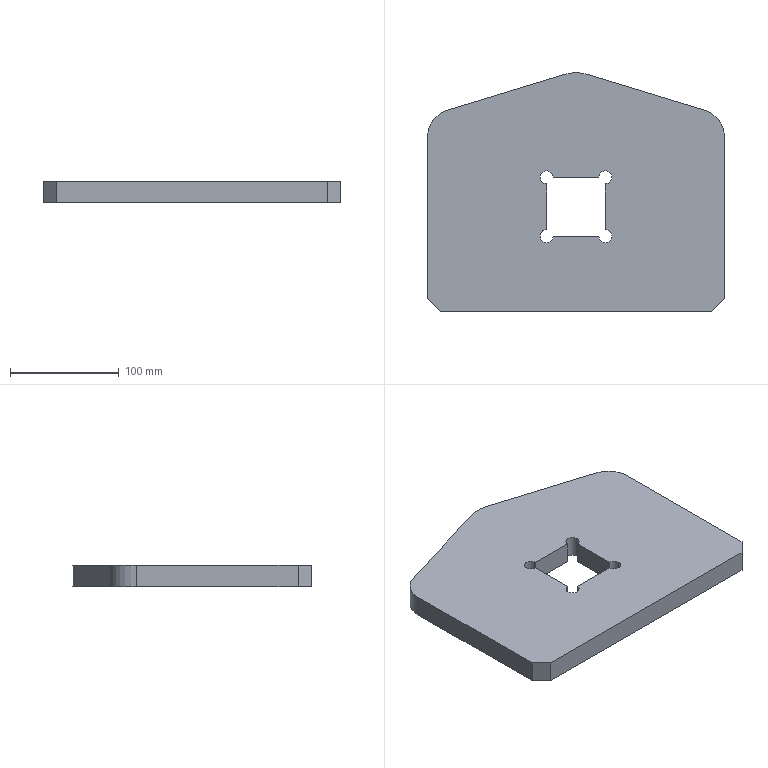Part | SolidWorks | features Extrusion 1 | 1 solid | 22 faces | box 273 x 219.3 x 20 mm | volume 1021205 mm3 | plane 13 | cylinder 9 | commonest cylinder face diameters 12 x6 50 x2 70 x1
STEP:
#1=CARTESIAN_POINT('',(-27.,75.,20.));
#2=VERTEX_POINT('',#1);
#3=CARTESIAN_POINT('',(-33.,69.,20.));
#4=VERTEX_POINT('',#3);
#5=CARTESIAN_POINT('',(-27.,69.,20.));
#6=DIRECTION('',(0.,0.,1.));
#7=DIRECTION('',(-1.,0.,0.));
#8=AXIS2_PLACEMENT_3D('',#5,#6,#7);
#9=CIRCLE('',#8,6.);
#10=EDGE_CURVE('',#2,#4,#9,.T.);
#11=ORIENTED_EDGE('',*,*,#10,.T.);
#12=CARTESIAN_POINT('',(-33.,69.,0.));
#13=VERTEX_POINT('',#12);
#14=CARTESIAN_POINT('',(-33.,69.,20.));
#15=DIRECTION('',(0.,0.,-1.));
#16=VECTOR('',#15,1000.);
#17=LINE('',#14,#16);
#18=EDGE_CURVE('',#4,#13,#17,.T.);
#19=ORIENTED_EDGE('',*,*,#18,.T.);
#20=CARTESIAN_POINT('',(-27.,75.,0.));
#21=VERTEX_POINT('',#20);
#22=CARTESIAN_POINT('',(-27.,69.,0.));
#23=DIRECTION('',(0.,0.,1.));
#24=DIRECTION('',(-1.,0.,0.));
#25=AXIS2_PLACEMENT_3D('',#22,#23,#24);
#26=CIRCLE('',#25,6.);
#27=EDGE_CURVE('',#21,#13,#26,.T.);
#28=ORIENTED_EDGE('',*,*,#27,.F.);
#29=CARTESIAN_POINT('',(-27.,75.,20.));
#30=DIRECTION('',(0.,0.,-1.));
#31=VECTOR('',#30,1000.);
#32=LINE('',#29,#31);
#33=EDGE_CURVE('',#2,#21,#32,.T.);
#34=ORIENTED_EDGE('',*,*,#33,.F.);
#35=EDGE_LOOP('',(#11,#19,#28,#34));
#36=FACE_OUTER_BOUND('',#35,.T.);
#37=CARTESIAN_POINT('',(-27.,69.,20.));
#38=DIRECTION('',(0.,0.,-1.));
#39=DIRECTION('',(-1.,0.,0.));
#40=AXIS2_PLACEMENT_3D('',#37,#38,#39);
#41=CYLINDRICAL_SURFACE('',#40,6.);
#42=ADVANCED_FACE('',(#36),#41,.F.);
#43=CARTESIAN_POINT('',(-21.,123.,20.));
#44=VERTEX_POINT('',#43);
#45=CARTESIAN_POINT('',(-33.,123.,20.));
#46=VERTEX_POINT('',#45);
#47=CARTESIAN_POINT('',(-27.,123.,20.));
#48=DIRECTION('',(0.,0.,1.));
#49=DIRECTION('',(-1.,0.,0.));
#50=AXIS2_PLACEMENT_3D('',#47,#48,#49);
#51=CIRCLE('',#50,6.);
#52=EDGE_CURVE('',#44,#46,#51,.T.);
#53=ORIENTED_EDGE('',*,*,#52,.T.);
#54=CARTESIAN_POINT('',(-33.,123.,0.));
#55=VERTEX_POINT('',#54);
#56=CARTESIAN_POINT('',(-33.,123.,20.));
#57=DIRECTION('',(0.,0.,-1.));
#58=VECTOR('',#57,1000.);
#59=LINE('',#56,#58);
#60=EDGE_CURVE('',#46,#55,#59,.T.);
#61=ORIENTED_EDGE('',*,*,#60,.T.);
#62=CARTESIAN_POINT('',(-21.,123.,0.));
#63=VERTEX_POINT('',#62);
#64=CARTESIAN_POINT('',(-27.,123.,0.));
#65=DIRECTION('',(0.,0.,1.));
#66=DIRECTION('',(-1.,0.,0.));
#67=AXIS2_PLACEMENT_3D('',#64,#65,#66);
#68=CIRCLE('',#67,6.);
#69=EDGE_CURVE('',#63,#55,#68,.T.);
#70=ORIENTED_EDGE('',*,*,#69,.F.);
#71=CARTESIAN_POINT('',(-21.,123.,20.));
#72=DIRECTION('',(0.,0.,-1.));
#73=VECTOR('',#72,1000.);
#74=LINE('',#71,#73);
#75=EDGE_CURVE('',#44,#63,#74,.T.);
#76=ORIENTED_EDGE('',*,*,#75,.F.);
#77=EDGE_LOOP('',(#53,#61,#70,#76));
#78=FACE_OUTER_BOUND('',#77,.T.);
#79=CARTESIAN_POINT('',(-27.,123.,20.));
#80=DIRECTION('',(0.,0.,-1.));
#81=DIRECTION('',(-1.,0.,0.));
#82=AXIS2_PLACEMENT_3D('',#79,#80,#81);
#83=CYLINDRICAL_SURFACE('',#82,6.);
#84=ADVANCED_FACE('',(#78),#83,.F.);
#85=CARTESIAN_POINT('',(124.5,0.,20.));
#86=VERTEX_POINT('',#85);
#87=CARTESIAN_POINT('',(136.5,12.,20.));
#88=VERTEX_POINT('',#87);
#89=CARTESIAN_POINT('',(124.5,0.,20.));
#90=DIRECTION('',(0.7071,0.7071,0.));
#91=VECTOR('',#90,1000.);
#92=LINE('',#89,#91);
#93=EDGE_CURVE('',#86,#88,#92,.T.);
#94=ORIENTED_EDGE('',*,*,#93,.T.);
#95=CARTESIAN_POINT('',(136.5,160.6,20.));
#96=VERTEX_POINT('',#95);
#97=CARTESIAN_POINT('',(136.5,12.,20.));
#98=DIRECTION('',(0.,1.,0.));
#99=VECTOR('',#98,1000.);
#100=LINE('',#97,#99);
#101=EDGE_CURVE('',#88,#96,#100,.T.);
#102=ORIENTED_EDGE('',*,*,#101,.T.);
#103=CARTESIAN_POINT('',(118.823,184.503,20.));
#104=VERTEX_POINT('',#103);
#105=CARTESIAN_POINT('',(111.5,160.6,20.));
#106=DIRECTION('',(0.,0.,1.));
#107=DIRECTION('',(1.,0.,0.));
#108=AXIS2_PLACEMENT_3D('',#105,#106,#107);
#109=CIRCLE('',#108,25.);
#110=EDGE_CURVE('',#96,#104,#109,.T.);
#111=ORIENTED_EDGE('',*,*,#110,.T.);
#112=CARTESIAN_POINT('',(10.252,217.765,20.));
#113=VERTEX_POINT('',#112);
#114=CARTESIAN_POINT('',(10.252,217.765,20.));
#115=DIRECTION('',(-0.9561,0.2929,0.));
#116=VECTOR('',#115,1000.);
#117=LINE('',#114,#116);
#118=EDGE_CURVE('',#104,#113,#117,.T.);
#119=ORIENTED_EDGE('',*,*,#118,.T.);
#120=CARTESIAN_POINT('',(-10.252,217.765,20.));
#121=VERTEX_POINT('',#120);
#122=CARTESIAN_POINT('',(0.,184.3,20.));
#123=DIRECTION('',(0.,0.,1.));
#124=DIRECTION('',(1.,0.,0.));
#125=AXIS2_PLACEMENT_3D('',#122,#123,#124);
#126=CIRCLE('',#125,35.);
#127=EDGE_CURVE('',#113,#121,#126,.T.);
#128=ORIENTED_EDGE('',*,*,#127,.T.);
#129=CARTESIAN_POINT('',(-118.823,184.503,20.));
#130=VERTEX_POINT('',#129);
#131=CARTESIAN_POINT('',(-10.252,217.765,20.));
#132=DIRECTION('',(-0.9561,-0.2929,0.));
#133=VECTOR('',#132,1000.);
#134=LINE('',#131,#133);
#135=EDGE_CURVE('',#121,#130,#134,.T.);
#136=ORIENTED_EDGE('',*,*,#135,.T.);
#137=CARTESIAN_POINT('',(-136.5,160.6,20.));
#138=VERTEX_POINT('',#137);
#139=CARTESIAN_POINT('',(-111.5,160.6,20.));
#140=DIRECTION('',(0.,0.,1.));
#141=DIRECTION('',(-1.,0.,0.));
#142=AXIS2_PLACEMENT_3D('',#139,#140,#141);
#143=CIRCLE('',#142,25.);
#144=EDGE_CURVE('',#130,#138,#143,.T.);
#145=ORIENTED_EDGE('',*,*,#144,.T.);
#146=CARTESIAN_POINT('',(-136.5,12.,20.));
#147=VERTEX_POINT('',#146);
#148=CARTESIAN_POINT('',(-136.5,12.,20.));
#149=DIRECTION('',(0.,-1.,0.));
#150=VECTOR('',#149,1000.);
#151=LINE('',#148,#150);
#152=EDGE_CURVE('',#138,#147,#151,.T.);
#153=ORIENTED_EDGE('',*,*,#152,.T.);
#154=CARTESIAN_POINT('',(-124.5,0.,20.));
#155=VERTEX_POINT('',#154);
#156=CARTESIAN_POINT('',(-124.5,0.,20.));
#157=DIRECTION('',(0.7071,-0.7071,0.));
#158=VECTOR('',#157,1000.);
#159=LINE('',#156,#158);
#160=EDGE_CURVE('',#147,#155,#159,.T.);
#161=ORIENTED_EDGE('',*,*,#160,.T.);
#162=CARTESIAN_POINT('',(-124.5,0.,20.));
#163=DIRECTION('',(1.,0.,0.));
#164=VECTOR('',#163,1000.);
#165=LINE('',#162,#164);
#166=EDGE_CURVE('',#155,#86,#165,.T.);
#167=ORIENTED_EDGE('',*,*,#166,.T.);
#168=EDGE_LOOP('',(#94,#102,#111,#119,#128,#136,#145,#153,#161,#167));
#169=FACE_OUTER_BOUND('',#168,.T.);
#170=CARTESIAN_POINT('',(27.,75.,20.));
#171=VERTEX_POINT('',#170);
#172=CARTESIAN_POINT('',(27.,117.,20.));
#173=VERTEX_POINT('',#172);
#174=CARTESIAN_POINT('',(27.,117.,20.));
#175=DIRECTION('',(0.,1.,0.));
#176=VECTOR('',#175,1000.);
#177=LINE('',#174,#176);
#178=EDGE_CURVE('',#171,#173,#177,.T.);
#179=ORIENTED_EDGE('',*,*,#178,.F.);
#180=CARTESIAN_POINT('',(21.,69.,20.));
#181=VERTEX_POINT('',#180);
#182=CARTESIAN_POINT('',(27.,69.,20.));
#183=DIRECTION('',(0.,0.,1.));
#184=DIRECTION('',(1.,0.,0.));
#185=AXIS2_PLACEMENT_3D('',#182,#183,#184);
#186=CIRCLE('',#185,6.);
#187=EDGE_CURVE('',#181,#171,#186,.T.);
#188=ORIENTED_EDGE('',*,*,#187,.F.);
#189=CARTESIAN_POINT('',(-21.,69.,20.));
#190=VERTEX_POINT('',#189);
#191=CARTESIAN_POINT('',(21.,69.,20.));
#192=DIRECTION('',(1.,0.,0.));
#193=VECTOR('',#192,1000.);
#194=LINE('',#191,#193);
#195=EDGE_CURVE('',#190,#181,#194,.T.);
#196=ORIENTED_EDGE('',*,*,#195,.F.);
#197=CARTESIAN_POINT('',(-27.,69.,20.));
#198=DIRECTION('',(0.,0.,1.));
#199=DIRECTION('',(-1.,0.,0.));
#200=AXIS2_PLACEMENT_3D('',#197,#198,#199);
#201=CIRCLE('',#200,6.);
#202=EDGE_CURVE('',#4,#190,#201,.T.);
#203=ORIENTED_EDGE('',*,*,#202,.F.);
#204=ORIENTED_EDGE('',*,*,#10,.F.);
#205=CARTESIAN_POINT('',(-27.,117.,20.));
#206=VERTEX_POINT('',#205);
#207=CARTESIAN_POINT('',(-27.,117.,20.));
#208=DIRECTION('',(0.,-1.,0.));
#209=VECTOR('',#208,1000.);
#210=LINE('',#207,#209);
#211=EDGE_CURVE('',#206,#2,#210,.T.);
#212=ORIENTED_EDGE('',*,*,#211,.F.);
#213=CARTESIAN_POINT('',(-27.,123.,20.));
#214=DIRECTION('',(0.,0.,1.));
#215=DIRECTION('',(-1.,0.,0.));
#216=AXIS2_PLACEMENT_3D('',#213,#214,#215);
#217=CIRCLE('',#216,6.);
#218=EDGE_CURVE('',#46,#206,#217,.T.);
#219=ORIENTED_EDGE('',*,*,#218,.F.);
#220=ORIENTED_EDGE('',*,*,#52,.F.);
#221=CARTESIAN_POINT('',(21.,123.,20.));
#222=VERTEX_POINT('',#221);
#223=CARTESIAN_POINT('',(-21.,123.,20.));
#224=DIRECTION('',(-1.,0.,0.));
#225=VECTOR('',#224,1000.);
#226=LINE('',#223,#225);
#227=EDGE_CURVE('',#222,#44,#226,.T.);
#228=ORIENTED_EDGE('',*,*,#227,.F.);
#229=CARTESIAN_POINT('',(27.,123.,20.));
#230=DIRECTION('',(0.,0.,1.));
#231=DIRECTION('',(1.,0.,0.));
#232=AXIS2_PLACEMENT_3D('',#229,#230,#231);
#233=CIRCLE('',#232,6.);
#234=EDGE_CURVE('',#173,#222,#233,.T.);
#235=ORIENTED_EDGE('',*,*,#234,.F.);
#236=EDGE_LOOP('',(#179,#188,#196,#203,#204,#212,#219,#220,#228,#235));
#237=FACE_BOUND('',#236,.T.);
#238=CARTESIAN_POINT('',(111.5,160.6,20.));
#239=DIRECTION('',(0.,0.,1.));
#240=DIRECTION('',(1.,0.,0.));
#241=AXIS2_PLACEMENT_3D('',#238,#239,#240);
#242=PLANE('',#241);
#243=ADVANCED_FACE('',(#169,#237),#242,.T.);
#244=CARTESIAN_POINT('',(124.5,0.,0.));
#245=VERTEX_POINT('',#244);
#246=CARTESIAN_POINT('',(136.5,12.,0.));
#247=VERTEX_POINT('',#246);
#248=CARTESIAN_POINT('',(124.5,0.,0.));
#249=DIRECTION('',(0.7071,0.7071,0.));
#250=VECTOR('',#249,1000.);
#251=LINE('',#248,#250);
#252=EDGE_CURVE('',#245,#247,#251,.T.);
#253=ORIENTED_EDGE('',*,*,#252,.F.);
#254=CARTESIAN_POINT('',(-124.5,0.,0.));
#255=VERTEX_POINT('',#254);
#256=CARTESIAN_POINT('',(-124.5,0.,0.));
#257=DIRECTION('',(1.,0.,0.));
#258=VECTOR('',#257,1000.);
#259=LINE('',#256,#258);
#260=EDGE_CURVE('',#255,#245,#259,.T.);
#261=ORIENTED_EDGE('',*,*,#260,.F.);
#262=CARTESIAN_POINT('',(-136.5,12.,0.));
#263=VERTEX_POINT('',#262);
#264=CARTESIAN_POINT('',(-124.5,0.,0.));
#265=DIRECTION('',(0.7071,-0.7071,0.));
#266=VECTOR('',#265,1000.);
#267=LINE('',#264,#266);
#268=EDGE_CURVE('',#263,#255,#267,.T.);
#269=ORIENTED_EDGE('',*,*,#268,.F.);
#270=CARTESIAN_POINT('',(-136.5,160.6,0.));
#271=VERTEX_POINT('',#270);
#272=CARTESIAN_POINT('',(-136.5,12.,0.));
#273=DIRECTION('',(0.,-1.,0.));
#274=VECTOR('',#273,1000.);
#275=LINE('',#272,#274);
#276=EDGE_CURVE('',#271,#263,#275,.T.);
#277=ORIENTED_EDGE('',*,*,#276,.F.);
#278=CARTESIAN_POINT('',(-118.823,184.503,0.));
#279=VERTEX_POINT('',#278);
#280=CARTESIAN_POINT('',(-111.5,160.6,0.));
#281=DIRECTION('',(0.,0.,1.));
#282=DIRECTION('',(-1.,0.,0.));
#283=AXIS2_PLACEMENT_3D('',#280,#281,#282);
#284=CIRCLE('',#283,25.);
#285=EDGE_CURVE('',#279,#271,#284,.T.);
#286=ORIENTED_EDGE('',*,*,#285,.F.);
#287=CARTESIAN_POINT('',(-10.252,217.765,0.));
#288=VERTEX_POINT('',#287);
#289=CARTESIAN_POINT('',(-10.252,217.765,0.));
#290=DIRECTION('',(-0.9561,-0.2929,0.));
#291=VECTOR('',#290,1000.);
#292=LINE('',#289,#291);
#293=EDGE_CURVE('',#288,#279,#292,.T.);
#294=ORIENTED_EDGE('',*,*,#293,.F.);
#295=CARTESIAN_POINT('',(10.252,217.765,0.));
#296=VERTEX_POINT('',#295);
#297=CARTESIAN_POINT('',(0.,184.3,0.));
#298=DIRECTION('',(0.,0.,1.));
#299=DIRECTION('',(1.,0.,0.));
#300=AXIS2_PLACEMENT_3D('',#297,#298,#299);
#301=CIRCLE('',#300,35.);
#302=EDGE_CURVE('',#296,#288,#301,.T.);
#303=ORIENTED_EDGE('',*,*,#302,.F.);
#304=CARTESIAN_POINT('',(118.823,184.503,0.));
#305=VERTEX_POINT('',#304);
#306=CARTESIAN_POINT('',(10.252,217.765,0.));
#307=DIRECTION('',(-0.9561,0.2929,0.));
#308=VECTOR('',#307,1000.);
#309=LINE('',#306,#308);
#310=EDGE_CURVE('',#305,#296,#309,.T.);
#311=ORIENTED_EDGE('',*,*,#310,.F.);
#312=CARTESIAN_POINT('',(136.5,160.6,0.));
#313=VERTEX_POINT('',#312);
#314=CARTESIAN_POINT('',(111.5,160.6,0.));
#315=DIRECTION('',(0.,0.,1.));
#316=DIRECTION('',(1.,0.,0.));
#317=AXIS2_PLACEMENT_3D('',#314,#315,#316);
#318=CIRCLE('',#317,25.);
#319=EDGE_CURVE('',#313,#305,#318,.T.);
#320=ORIENTED_EDGE('',*,*,#319,.F.);
#321=CARTESIAN_POINT('',(136.5,12.,0.));
#322=DIRECTION('',(0.,1.,0.));
#323=VECTOR('',#322,1000.);
#324=LINE('',#321,#323);
#325=EDGE_CURVE('',#247,#313,#324,.T.);
#326=ORIENTED_EDGE('',*,*,#325,.F.);
#327=EDGE_LOOP('',(#253,#261,#269,#277,#286,#294,#303,#311,#320,#326));
#328=FACE_OUTER_BOUND('',#327,.T.);
#329=CARTESIAN_POINT('',(21.,69.,0.));
#330=VERTEX_POINT('',#329);
#331=CARTESIAN_POINT('',(27.,75.,0.));
#332=VERTEX_POINT('',#331);
#333=CARTESIAN_POINT('',(27.,69.,0.));
#334=DIRECTION('',(0.,0.,1.));
#335=DIRECTION('',(1.,0.,0.));
#336=AXIS2_PLACEMENT_3D('',#333,#334,#335);
#337=CIRCLE('',#336,6.);
#338=EDGE_CURVE('',#330,#332,#337,.T.);
#339=ORIENTED_EDGE('',*,*,#338,.T.);
#340=CARTESIAN_POINT('',(27.,117.,0.));
#341=VERTEX_POINT('',#340);
#342=CARTESIAN_POINT('',(27.,117.,0.));
#343=DIRECTION('',(0.,1.,0.));
#344=VECTOR('',#343,1000.);
#345=LINE('',#342,#344);
#346=EDGE_CURVE('',#332,#341,#345,.T.);
#347=ORIENTED_EDGE('',*,*,#346,.T.);
#348=CARTESIAN_POINT('',(21.,123.,0.));
#349=VERTEX_POINT('',#348);
#350=CARTESIAN_POINT('',(27.,123.,0.));
#351=DIRECTION('',(0.,0.,1.));
#352=DIRECTION('',(1.,0.,0.));
#353=AXIS2_PLACEMENT_3D('',#350,#351,#352);
#354=CIRCLE('',#353,6.);
#355=EDGE_CURVE('',#341,#349,#354,.T.);
#356=ORIENTED_EDGE('',*,*,#355,.T.);
#357=CARTESIAN_POINT('',(-21.,123.,0.));
#358=DIRECTION('',(-1.,0.,0.));
#359=VECTOR('',#358,1000.);
#360=LINE('',#357,#359);
#361=EDGE_CURVE('',#349,#63,#360,.T.);
#362=ORIENTED_EDGE('',*,*,#361,.T.);
#363=ORIENTED_EDGE('',*,*,#69,.T.);
#364=CARTESIAN_POINT('',(-27.,117.,0.));
#365=VERTEX_POINT('',#364);
#366=CARTESIAN_POINT('',(-27.,123.,0.));
#367=DIRECTION('',(0.,0.,1.));
#368=DIRECTION('',(-1.,0.,0.));
#369=AXIS2_PLACEMENT_3D('',#366,#367,#368);
#370=CIRCLE('',#369,6.);
#371=EDGE_CURVE('',#55,#365,#370,.T.);
#372=ORIENTED_EDGE('',*,*,#371,.T.);
#373=CARTESIAN_POINT('',(-27.,117.,0.));
#374=DIRECTION('',(0.,-1.,0.));
#375=VECTOR('',#374,1000.);
#376=LINE('',#373,#375);
#377=EDGE_CURVE('',#365,#21,#376,.T.);
#378=ORIENTED_EDGE('',*,*,#377,.T.);
#379=ORIENTED_EDGE('',*,*,#27,.T.);
#380=CARTESIAN_POINT('',(-21.,69.,0.));
#381=VERTEX_POINT('',#380);
#382=CARTESIAN_POINT('',(-27.,69.,0.));
#383=DIRECTION('',(0.,0.,1.));
#384=DIRECTION('',(-1.,0.,0.));
#385=AXIS2_PLACEMENT_3D('',#382,#383,#384);
#386=CIRCLE('',#385,6.);
#387=EDGE_CURVE('',#13,#381,#386,.T.);
#388=ORIENTED_EDGE('',*,*,#387,.T.);
#389=CARTESIAN_POINT('',(21.,69.,0.));
#390=DIRECTION('',(1.,0.,0.));
#391=VECTOR('',#390,1000.);
#392=LINE('',#389,#391);
#393=EDGE_CURVE('',#381,#330,#392,.T.);
#394=ORIENTED_EDGE('',*,*,#393,.T.);
#395=EDGE_LOOP('',(#339,#347,#356,#362,#363,#372,#378,#379,#388,#394));
#396=FACE_BOUND('',#395,.T.);
#397=CARTESIAN_POINT('',(111.5,160.6,0.));
#398=DIRECTION('',(0.,0.,1.));
#399=DIRECTION('',(1.,0.,0.));
#400=AXIS2_PLACEMENT_3D('',#397,#398,#399);
#401=PLANE('',#400);
#402=ADVANCED_FACE('',(#328,#396),#401,.F.);
#403=ORIENTED_EDGE('',*,*,#252,.T.);
#404=CARTESIAN_POINT('',(136.5,12.,20.));
#405=DIRECTION('',(0.,0.,-1.));
#406=VECTOR('',#405,1000.);
#407=LINE('',#404,#406);
#408=EDGE_CURVE('',#88,#247,#407,.T.);
#409=ORIENTED_EDGE('',*,*,#408,.F.);
#410=ORIENTED_EDGE('',*,*,#93,.F.);
#411=CARTESIAN_POINT('',(124.5,0.,20.));
#412=DIRECTION('',(0.,0.,-1.));
#413=VECTOR('',#412,1000.);
#414=LINE('',#411,#413);
#415=EDGE_CURVE('',#86,#245,#414,.T.);
#416=ORIENTED_EDGE('',*,*,#415,.T.);
#417=EDGE_LOOP('',(#403,#409,#410,#416));
#418=FACE_OUTER_BOUND('',#417,.T.);
#419=CARTESIAN_POINT('',(124.5,0.,20.));
#420=DIRECTION('',(-0.7071,0.7071,0.));
#421=DIRECTION('',(-0.7071,-0.7071,0.));
#422=AXIS2_PLACEMENT_3D('',#419,#420,#421);
#423=PLANE('',#422);
#424=ADVANCED_FACE('',(#418),#423,.F.);
#425=ORIENTED_EDGE('',*,*,#325,.T.);
#426=CARTESIAN_POINT('',(136.5,160.6,20.));
#427=DIRECTION('',(0.,0.,-1.));
#428=VECTOR('',#427,1000.);
#429=LINE('',#426,#428);
#430=EDGE_CURVE('',#96,#313,#429,.T.);
#431=ORIENTED_EDGE('',*,*,#430,.F.);
#432=ORIENTED_EDGE('',*,*,#101,.F.);
#433=ORIENTED_EDGE('',*,*,#408,.T.);
#434=EDGE_LOOP('',(#425,#431,#432,#433));
#435=FACE_OUTER_BOUND('',#434,.T.);
#436=CARTESIAN_POINT('',(136.5,12.,20.));
#437=DIRECTION('',(-1.,0.,0.));
#438=DIRECTION('',(0.,0.,1.));
#439=AXIS2_PLACEMENT_3D('',#436,#437,#438);
#440=PLANE('',#439);
#441=ADVANCED_FACE('',(#435),#440,.F.);
#442=ORIENTED_EDGE('',*,*,#319,.T.);
#443=CARTESIAN_POINT('',(118.823,184.503,20.));
#444=DIRECTION('',(0.,0.,-1.));
#445=VECTOR('',#444,1000.);
#446=LINE('',#443,#445);
#447=EDGE_CURVE('',#104,#305,#446,.T.);
#448=ORIENTED_EDGE('',*,*,#447,.F.);
#449=ORIENTED_EDGE('',*,*,#110,.F.);
#450=ORIENTED_EDGE('',*,*,#430,.T.);
#451=EDGE_LOOP('',(#442,#448,#449,#450));
#452=FACE_OUTER_BOUND('',#451,.T.);
#453=CARTESIAN_POINT('',(111.5,160.6,20.));
#454=DIRECTION('',(0.,0.,-1.));
#455=DIRECTION('',(-1.,0.,0.));
#456=AXIS2_PLACEMENT_3D('',#453,#454,#455);
#457=CYLINDRICAL_SURFACE('',#456,25.);
#458=ADVANCED_FACE('',(#452),#457,.T.);
#459=ORIENTED_EDGE('',*,*,#310,.T.);
#460=CARTESIAN_POINT('',(10.252,217.765,20.));
#461=DIRECTION('',(0.,0.,-1.));
#462=VECTOR('',#461,1000.);
#463=LINE('',#460,#462);
#464=EDGE_CURVE('',#113,#296,#463,.T.);
#465=ORIENTED_EDGE('',*,*,#464,.F.);
#466=ORIENTED_EDGE('',*,*,#118,.F.);
#467=ORIENTED_EDGE('',*,*,#447,.T.);
#468=EDGE_LOOP('',(#459,#465,#466,#467));
#469=FACE_OUTER_BOUND('',#468,.T.);
#470=CARTESIAN_POINT('',(10.252,217.765,20.));
#471=DIRECTION('',(-0.2929,-0.9561,0.));
#472=DIRECTION('',(0.9561,-0.2929,0.));
#473=AXIS2_PLACEMENT_3D('',#470,#471,#472);
#474=PLANE('',#473);
#475=ADVANCED_FACE('',(#469),#474,.F.);
#476=ORIENTED_EDGE('',*,*,#302,.T.);
#477=CARTESIAN_POINT('',(-10.252,217.765,20.));
#478=DIRECTION('',(0.,0.,-1.));
#479=VECTOR('',#478,1000.);
#480=LINE('',#477,#479);
#481=EDGE_CURVE('',#121,#288,#480,.T.);
#482=ORIENTED_EDGE('',*,*,#481,.F.);
#483=ORIENTED_EDGE('',*,*,#127,.F.);
#484=ORIENTED_EDGE('',*,*,#464,.T.);
#485=EDGE_LOOP('',(#476,#482,#483,#484));
#486=FACE_OUTER_BOUND('',#485,.T.);
#487=CARTESIAN_POINT('',(0.,184.3,20.));
#488=DIRECTION('',(0.,0.,-1.));
#489=DIRECTION('',(-1.,0.,0.));
#490=AXIS2_PLACEMENT_3D('',#487,#488,#489);
#491=CYLINDRICAL_SURFACE('',#490,35.);
#492=ADVANCED_FACE('',(#486),#491,.T.);
#493=ORIENTED_EDGE('',*,*,#293,.T.);
#494=CARTESIAN_POINT('',(-118.823,184.503,20.));
#495=DIRECTION('',(0.,0.,-1.));
#496=VECTOR('',#495,1000.);
#497=LINE('',#494,#496);
#498=EDGE_CURVE('',#130,#279,#497,.T.);
#499=ORIENTED_EDGE('',*,*,#498,.F.);
#500=ORIENTED_EDGE('',*,*,#135,.F.);
#501=ORIENTED_EDGE('',*,*,#481,.T.);
#502=EDGE_LOOP('',(#493,#499,#500,#501));
#503=FACE_OUTER_BOUND('',#502,.T.);
#504=CARTESIAN_POINT('',(-10.252,217.765,20.));
#505=DIRECTION('',(0.2929,-0.9561,0.));
#506=DIRECTION('',(0.9561,0.2929,0.));
#507=AXIS2_PLACEMENT_3D('',#504,#505,#506);
#508=PLANE('',#507);
#509=ADVANCED_FACE('',(#503),#508,.F.);
#510=ORIENTED_EDGE('',*,*,#285,.T.);
#511=CARTESIAN_POINT('',(-136.5,160.6,20.));
#512=DIRECTION('',(0.,0.,-1.));
#513=VECTOR('',#512,1000.);
#514=LINE('',#511,#513);
#515=EDGE_CURVE('',#138,#271,#514,.T.);
#516=ORIENTED_EDGE('',*,*,#515,.F.);
#517=ORIENTED_EDGE('',*,*,#144,.F.);
#518=ORIENTED_EDGE('',*,*,#498,.T.);
#519=EDGE_LOOP('',(#510,#516,#517,#518));
#520=FACE_OUTER_BOUND('',#519,.T.);
#521=CARTESIAN_POINT('',(-111.5,160.6,20.));
#522=DIRECTION('',(0.,0.,-1.));
#523=DIRECTION('',(-1.,0.,0.));
#524=AXIS2_PLACEMENT_3D('',#521,#522,#523);
#525=CYLINDRICAL_SURFACE('',#524,25.);
#526=ADVANCED_FACE('',(#520),#525,.T.);
#527=ORIENTED_EDGE('',*,*,#276,.T.);
#528=CARTESIAN_POINT('',(-136.5,12.,20.));
#529=DIRECTION('',(0.,0.,-1.));
#530=VECTOR('',#529,1000.);
#531=LINE('',#528,#530);
#532=EDGE_CURVE('',#147,#263,#531,.T.);
#533=ORIENTED_EDGE('',*,*,#532,.F.);
#534=ORIENTED_EDGE('',*,*,#152,.F.);
#535=ORIENTED_EDGE('',*,*,#515,.T.);
#536=EDGE_LOOP('',(#527,#533,#534,#535));
#537=FACE_OUTER_BOUND('',#536,.T.);
#538=CARTESIAN_POINT('',(-136.5,12.,20.));
#539=DIRECTION('',(1.,0.,0.));
#540=DIRECTION('',(0.,0.,-1.));
#541=AXIS2_PLACEMENT_3D('',#538,#539,#540);
#542=PLANE('',#541);
#543=ADVANCED_FACE('',(#537),#542,.F.);
#544=ORIENTED_EDGE('',*,*,#268,.T.);
#545=CARTESIAN_POINT('',(-124.5,0.,20.));
#546=DIRECTION('',(0.,0.,-1.));
#547=VECTOR('',#546,1000.);
#548=LINE('',#545,#547);
#549=EDGE_CURVE('',#155,#255,#548,.T.);
#550=ORIENTED_EDGE('',*,*,#549,.F.);
#551=ORIENTED_EDGE('',*,*,#160,.F.);
#552=ORIENTED_EDGE('',*,*,#532,.T.);
#553=EDGE_LOOP('',(#544,#550,#551,#552));
#554=FACE_OUTER_BOUND('',#553,.T.);
#555=CARTESIAN_POINT('',(-124.5,0.,20.));
#556=DIRECTION('',(0.7071,0.7071,0.));
#557=DIRECTION('',(-0.7071,0.7071,0.));
#558=AXIS2_PLACEMENT_3D('',#555,#556,#557);
#559=PLANE('',#558);
#560=ADVANCED_FACE('',(#554),#559,.F.);
#561=ORIENTED_EDGE('',*,*,#260,.T.);
#562=ORIENTED_EDGE('',*,*,#415,.F.);
#563=ORIENTED_EDGE('',*,*,#166,.F.);
#564=ORIENTED_EDGE('',*,*,#549,.T.);
#565=EDGE_LOOP('',(#561,#562,#563,#564));
#566=FACE_OUTER_BOUND('',#565,.T.);
#567=CARTESIAN_POINT('',(-124.5,0.,20.));
#568=DIRECTION('',(0.,1.,0.));
#569=DIRECTION('',(0.,0.,1.));
#570=AXIS2_PLACEMENT_3D('',#567,#568,#569);
#571=PLANE('',#570);
#572=ADVANCED_FACE('',(#566),#571,.F.);
#573=ORIENTED_EDGE('',*,*,#338,.F.);
#574=CARTESIAN_POINT('',(21.,69.,20.));
#575=DIRECTION('',(0.,0.,-1.));
#576=VECTOR('',#575,1000.);
#577=LINE('',#574,#576);
#578=EDGE_CURVE('',#181,#330,#577,.T.);
#579=ORIENTED_EDGE('',*,*,#578,.F.);
#580=ORIENTED_EDGE('',*,*,#187,.T.);
#581=CARTESIAN_POINT('',(27.,75.,20.));
#582=DIRECTION('',(0.,0.,-1.));
#583=VECTOR('',#582,1000.);
#584=LINE('',#581,#583);
#585=EDGE_CURVE('',#171,#332,#584,.T.);
#586=ORIENTED_EDGE('',*,*,#585,.T.);
#587=EDGE_LOOP('',(#573,#579,#580,#586));
#588=FACE_OUTER_BOUND('',#587,.T.);
#589=CARTESIAN_POINT('',(27.,69.,20.));
#590=DIRECTION('',(0.,0.,-1.));
#591=DIRECTION('',(-1.,0.,0.));
#592=AXIS2_PLACEMENT_3D('',#589,#590,#591);
#593=CYLINDRICAL_SURFACE('',#592,6.);
#594=ADVANCED_FACE('',(#588),#593,.F.);
#595=ORIENTED_EDGE('',*,*,#346,.F.);
#596=ORIENTED_EDGE('',*,*,#585,.F.);
#597=ORIENTED_EDGE('',*,*,#178,.T.);
#598=CARTESIAN_POINT('',(27.,117.,20.));
#599=DIRECTION('',(0.,0.,-1.));
#600=VECTOR('',#599,1000.);
#601=LINE('',#598,#600);
#602=EDGE_CURVE('',#173,#341,#601,.T.);
#603=ORIENTED_EDGE('',*,*,#602,.T.);
#604=EDGE_LOOP('',(#595,#596,#597,#603));
#605=FACE_OUTER_BOUND('',#604,.T.);
#606=CARTESIAN_POINT('',(27.,117.,20.));
#607=DIRECTION('',(-1.,0.,0.));
#608=DIRECTION('',(0.,-1.,0.));
#609=AXIS2_PLACEMENT_3D('',#606,#607,#608);
#610=PLANE('',#609);
#611=ADVANCED_FACE('',(#605),#610,.T.);
#612=ORIENTED_EDGE('',*,*,#355,.F.);
#613=ORIENTED_EDGE('',*,*,#602,.F.);
#614=ORIENTED_EDGE('',*,*,#234,.T.);
#615=CARTESIAN_POINT('',(21.,123.,20.));
#616=DIRECTION('',(0.,0.,-1.));
#617=VECTOR('',#616,1000.);
#618=LINE('',#615,#617);
#619=EDGE_CURVE('',#222,#349,#618,.T.);
#620=ORIENTED_EDGE('',*,*,#619,.T.);
#621=EDGE_LOOP('',(#612,#613,#614,#620));
#622=FACE_OUTER_BOUND('',#621,.T.);
#623=CARTESIAN_POINT('',(27.,123.,20.));
#624=DIRECTION('',(0.,0.,-1.));
#625=DIRECTION('',(-1.,0.,0.));
#626=AXIS2_PLACEMENT_3D('',#623,#624,#625);
#627=CYLINDRICAL_SURFACE('',#626,6.);
#628=ADVANCED_FACE('',(#622),#627,.F.);
#629=ORIENTED_EDGE('',*,*,#361,.F.);
#630=ORIENTED_EDGE('',*,*,#619,.F.);
#631=ORIENTED_EDGE('',*,*,#227,.T.);
#632=ORIENTED_EDGE('',*,*,#75,.T.);
#633=EDGE_LOOP('',(#629,#630,#631,#632));
#634=FACE_OUTER_BOUND('',#633,.T.);
#635=CARTESIAN_POINT('',(-21.,123.,20.));
#636=DIRECTION('',(0.,-1.,0.));
#637=DIRECTION('',(0.,0.,-1.));
#638=AXIS2_PLACEMENT_3D('',#635,#636,#637);
#639=PLANE('',#638);
#640=ADVANCED_FACE('',(#634),#639,.T.);
#641=ORIENTED_EDGE('',*,*,#60,.F.);
#642=ORIENTED_EDGE('',*,*,#218,.T.);
#643=CARTESIAN_POINT('',(-27.,117.,20.));
#644=DIRECTION('',(0.,0.,-1.));
#645=VECTOR('',#644,1000.);
#646=LINE('',#643,#645);
#647=EDGE_CURVE('',#206,#365,#646,.T.);
#648=ORIENTED_EDGE('',*,*,#647,.T.);
#649=ORIENTED_EDGE('',*,*,#371,.F.);
#650=EDGE_LOOP('',(#641,#642,#648,#649));
#651=FACE_OUTER_BOUND('',#650,.T.);
#652=CARTESIAN_POINT('',(-27.,123.,20.));
#653=DIRECTION('',(0.,0.,-1.));
#654=DIRECTION('',(-1.,0.,0.));
#655=AXIS2_PLACEMENT_3D('',#652,#653,#654);
#656=CYLINDRICAL_SURFACE('',#655,6.);
#657=ADVANCED_FACE('',(#651),#656,.F.);
#658=ORIENTED_EDGE('',*,*,#377,.F.);
#659=ORIENTED_EDGE('',*,*,#647,.F.);
#660=ORIENTED_EDGE('',*,*,#211,.T.);
#661=ORIENTED_EDGE('',*,*,#33,.T.);
#662=EDGE_LOOP('',(#658,#659,#660,#661));
#663=FACE_OUTER_BOUND('',#662,.T.);
#664=CARTESIAN_POINT('',(-27.,117.,20.));
#665=DIRECTION('',(1.,0.,0.));
#666=DIRECTION('',(0.,1.,0.));
#667=AXIS2_PLACEMENT_3D('',#664,#665,#666);
#668=PLANE('',#667);
#669=ADVANCED_FACE('',(#663),#668,.T.);
#670=ORIENTED_EDGE('',*,*,#18,.F.);
#671=ORIENTED_EDGE('',*,*,#202,.T.);
#672=CARTESIAN_POINT('',(-21.,69.,20.));
#673=DIRECTION('',(0.,0.,-1.));
#674=VECTOR('',#673,1000.);
#675=LINE('',#672,#674);
#676=EDGE_CURVE('',#190,#381,#675,.T.);
#677=ORIENTED_EDGE('',*,*,#676,.T.);
#678=ORIENTED_EDGE('',*,*,#387,.F.);
#679=EDGE_LOOP('',(#670,#671,#677,#678));
#680=FACE_OUTER_BOUND('',#679,.T.);
#681=CARTESIAN_POINT('',(-27.,69.,20.));
#682=DIRECTION('',(0.,0.,-1.));
#683=DIRECTION('',(-1.,0.,0.));
#684=AXIS2_PLACEMENT_3D('',#681,#682,#683);
#685=CYLINDRICAL_SURFACE('',#684,6.);
#686=ADVANCED_FACE('',(#680),#685,.F.);
#687=ORIENTED_EDGE('',*,*,#393,.F.);
#688=ORIENTED_EDGE('',*,*,#676,.F.);
#689=ORIENTED_EDGE('',*,*,#195,.T.);
#690=ORIENTED_EDGE('',*,*,#578,.T.);
#691=EDGE_LOOP('',(#687,#688,#689,#690));
#692=FACE_OUTER_BOUND('',#691,.T.);
#693=CARTESIAN_POINT('',(21.,69.,20.));
#694=DIRECTION('',(0.,1.,0.));
#695=DIRECTION('',(0.,0.,1.));
#696=AXIS2_PLACEMENT_3D('',#693,#694,#695);
#697=PLANE('',#696);
#698=ADVANCED_FACE('',(#692),#697,.T.);
#699=CLOSED_SHELL('',(#42,#84,#243,#402,#424,#441,#458,#475,#492,#509,#526,#543,#560,#572,#594,#611,#628,#640,#657,#669,#686,#698));
#700=MANIFOLD_SOLID_BREP('',#699);
#701=CARTESIAN_POINT('',(0.,0.,0.));
#702=DIRECTION('',(0.,0.,1.));
#703=DIRECTION('',(1.,0.,0.));
#704=AXIS2_PLACEMENT_3D('',#701,#702,#703);
#705=(LENGTH_UNIT()NAMED_UNIT(*)SI_UNIT(.MILLI.,.METRE.));
#706=UNCERTAINTY_MEASURE_WITH_UNIT(LENGTH_MEASURE(0.00001),#705,'','');
#707=(NAMED_UNIT(*)PLANE_ANGLE_UNIT()SI_UNIT($,.RADIAN.));
#708=(NAMED_UNIT(*)SI_UNIT($,.STERADIAN.)SOLID_ANGLE_UNIT());
#709=(GEOMETRIC_REPRESENTATION_CONTEXT(3)GLOBAL_UNCERTAINTY_ASSIGNED_CONTEXT((#706))GLOBAL_UNIT_ASSIGNED_CONTEXT((#705,#707,#708))REPRESENTATION_CONTEXT('',''));
#710=ADVANCED_BREP_SHAPE_REPRESENTATION('',(#700,#704),#709);